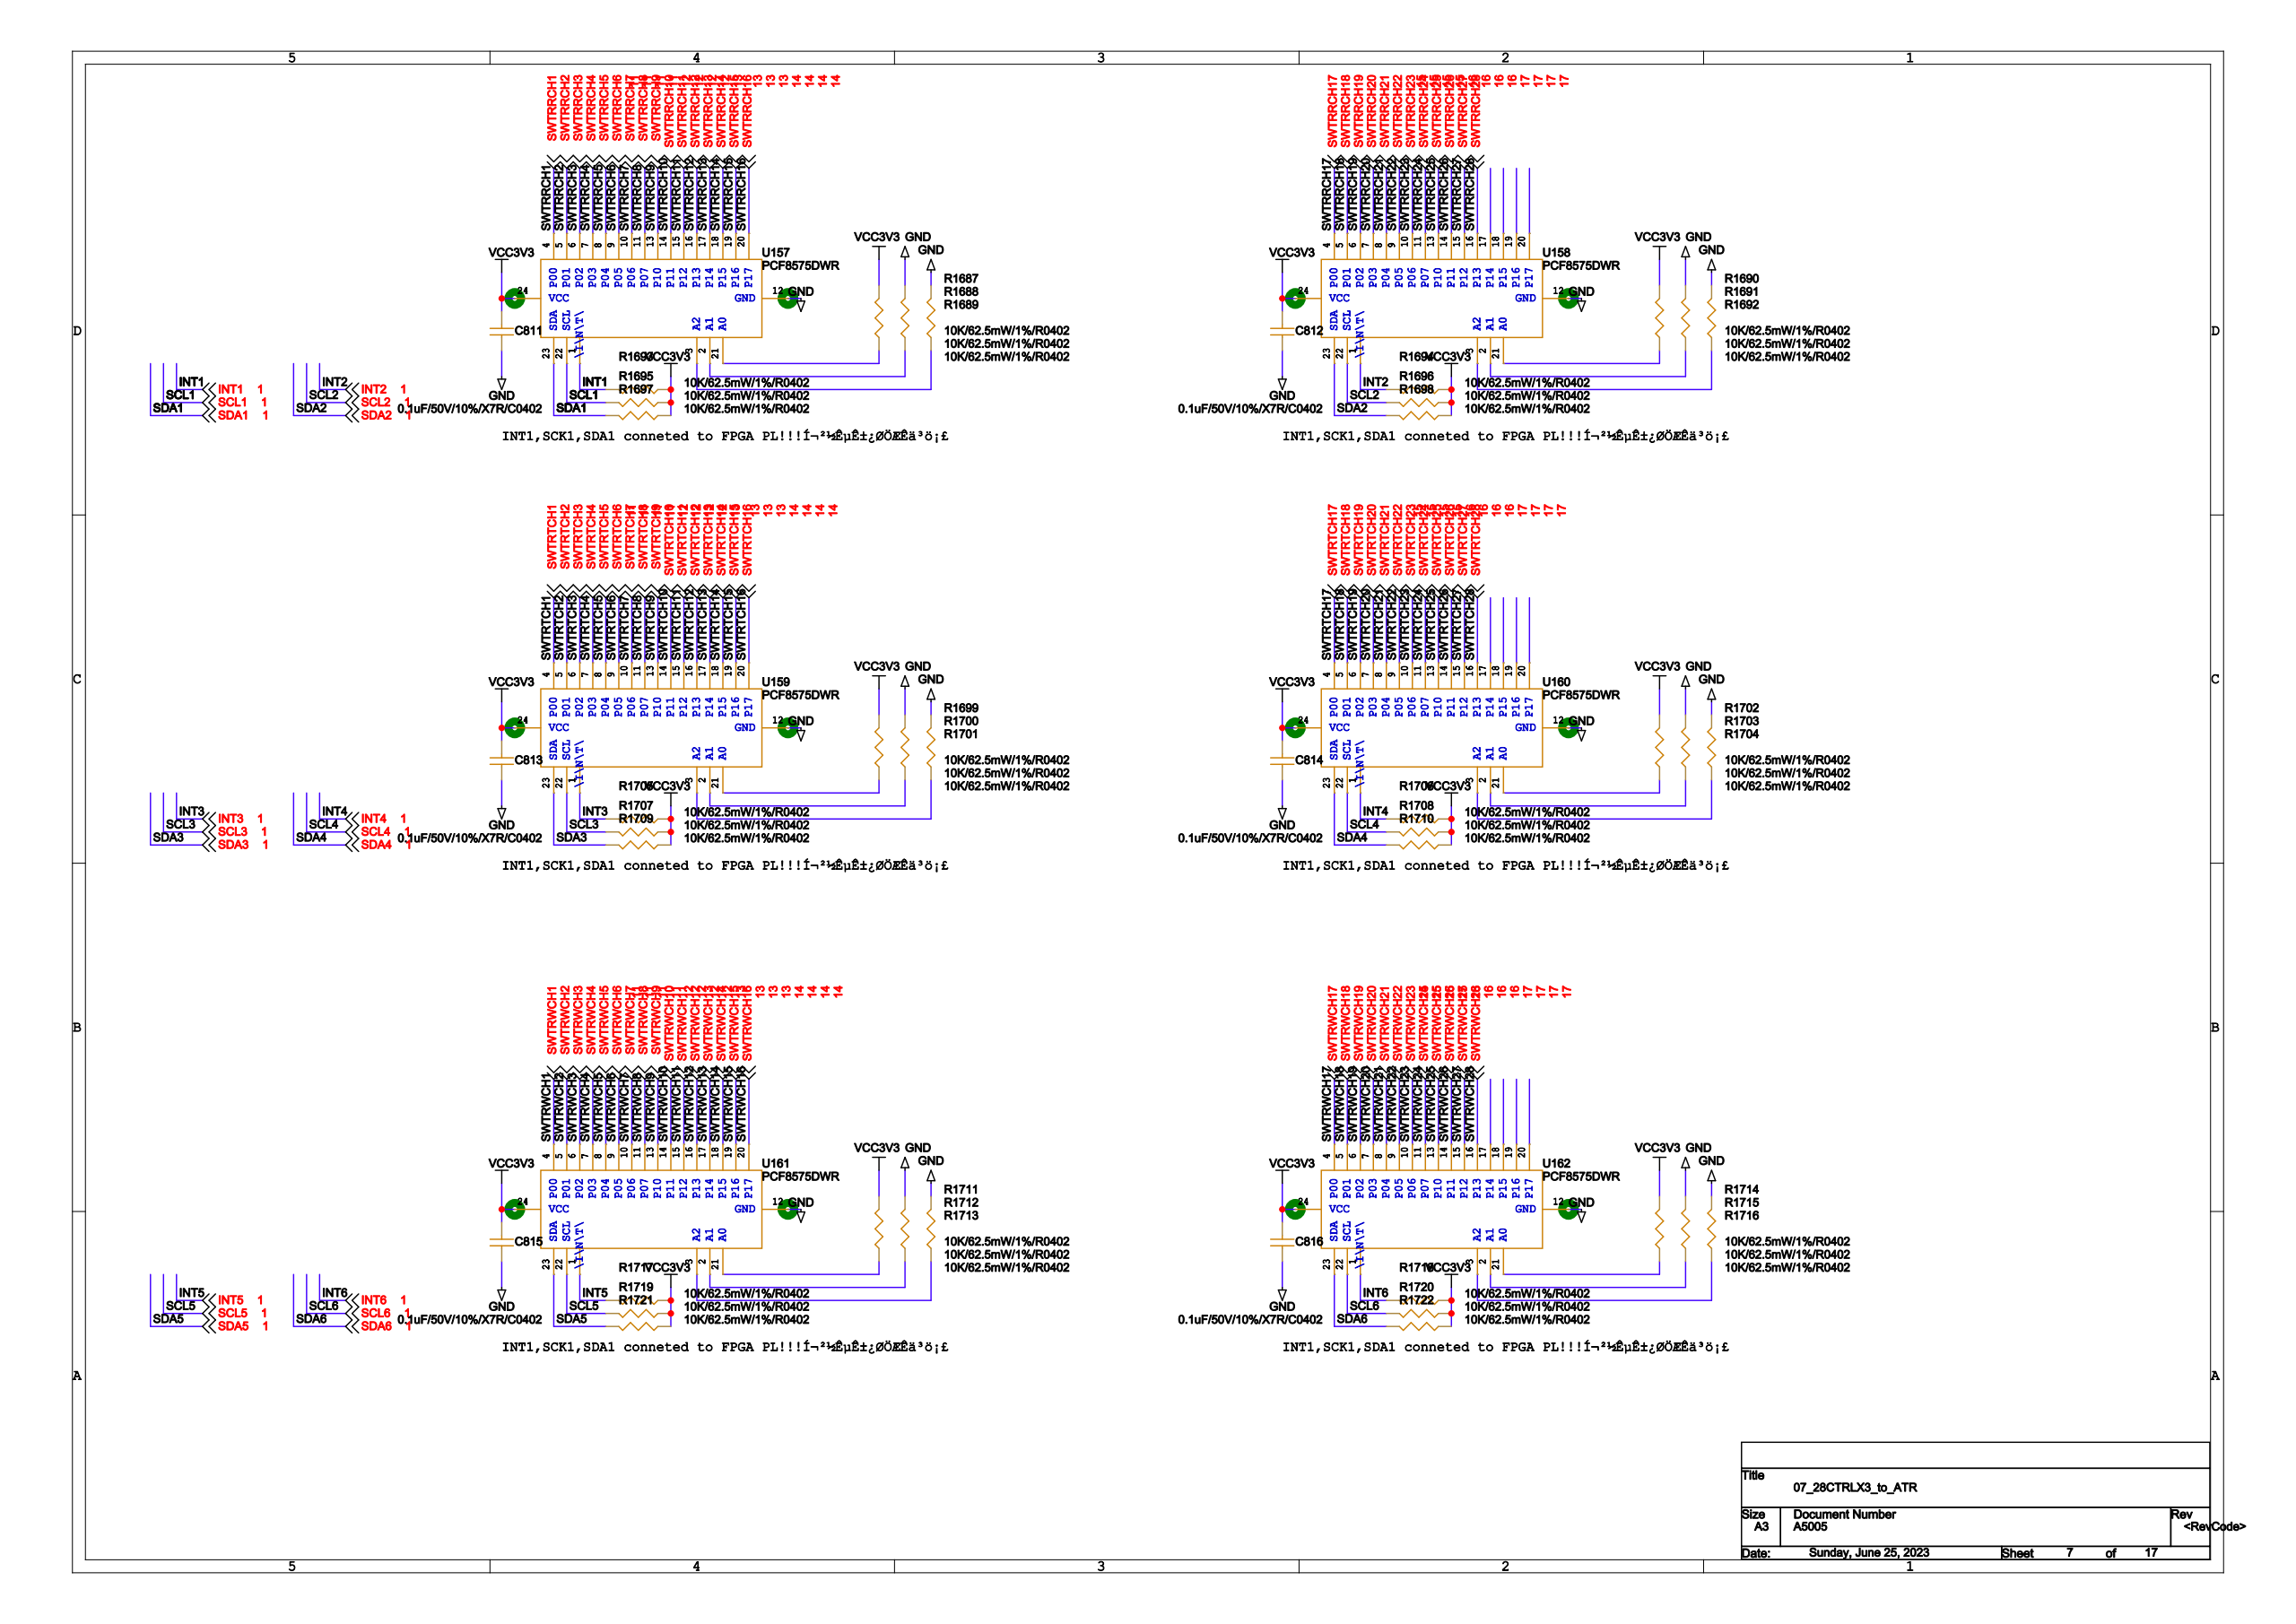Circuit board | Cadence Allegro | 1997 parts | 1536 nets | one sheet of the schematic
Parts on this sheet (reference | value | footprint):
C811 | 0.1uF/50V/10%/X7R/C0402 | 0402
C812 | 0.1uF/50V/10%/X7R/C0402 | 0402
C813 | 0.1uF/50V/10%/X7R/C0402 | 0402
C814 | 0.1uF/50V/10%/X7R/C0402 | 0402
C815 | 0.1uF/50V/10%/X7R/C0402 | 0402
C816 | 0.1uF/50V/10%/X7R/C0402 | 0402
R1687 | 10K/62.5mW/1%/R0402 | 0402
R1688 | 10K/62.5mW/1%/R0402 | 0402
R1689 | 10K/62.5mW/1%/R0402 | 0402
R1690 | 10K/62.5mW/1%/R0402 | 0402
R1691 | 10K/62.5mW/1%/R0402 | 0402
R1692 | 10K/62.5mW/1%/R0402 | 0402
R1693 | 10K/62.5mW/1%/R0402 | 0402
R1694 | 10K/62.5mW/1%/R0402 | 0402
R1695 | 10K/62.5mW/1%/R0402 | 0402
R1696 | 10K/62.5mW/1%/R0402 | 0402
R1697 | 10K/62.5mW/1%/R0402 | 0402
R1698 | 10K/62.5mW/1%/R0402 | 0402
R1699 | 10K/62.5mW/1%/R0402 | 0402
R1700 | 10K/62.5mW/1%/R0402 | 0402
R1701 | 10K/62.5mW/1%/R0402 | 0402
R1702 | 10K/62.5mW/1%/R0402 | 0402
R1703 | 10K/62.5mW/1%/R0402 | 0402
R1704 | 10K/62.5mW/1%/R0402 | 0402
R1705 | 10K/62.5mW/1%/R0402 | 0402
R1706 | 10K/62.5mW/1%/R0402 | 0402
R1707 | 10K/62.5mW/1%/R0402 | 0402
R1708 | 10K/62.5mW/1%/R0402 | 0402
R1709 | 10K/62.5mW/1%/R0402 | 0402
R1710 | 10K/62.5mW/1%/R0402 | 0402
R1711 | 10K/62.5mW/1%/R0402 | 0402
R1712 | 10K/62.5mW/1%/R0402 | 0402
R1713 | 10K/62.5mW/1%/R0402 | 0402
R1714 | 10K/62.5mW/1%/R0402 | 0402
R1715 | 10K/62.5mW/1%/R0402 | 0402
R1716 | 10K/62.5mW/1%/R0402 | 0402
R1717 | 10K/62.5mW/1%/R0402 | 0402
R1718 | 10K/62.5mW/1%/R0402 | 0402
R1719 | 10K/62.5mW/1%/R0402 | 0402
R1720 | 10K/62.5mW/1%/R0402 | 0402
R1721 | 10K/62.5mW/1%/R0402 | 0402
R1722 | 10K/62.5mW/1%/R0402 | 0402
U157 | PCF8575DWR | SOIC_24
U158 | PCF8575DWR | SOIC_24
U159 | PCF8575DWR | SOIC_24
U160 | PCF8575DWR | SOIC_24
U161 | PCF8575DWR | SOIC_24
U162 | PCF8575DWR | SOIC_24
Nets of these parts (net: part-pin ...):
3.3V: C811-2 C812-2 C813-2 C814-2 C815-2 C816-2 R1687-1 R1690-1 R1693-2 R1694-2 R1695-2 R1696-2 R1697-2 R1698-2 R1699-1 R1702-1 R1705-2 R1706-2 R1707-2 R1708-2 R1709-2 R1710-2 R1711-1 R1714-1 R1717-2 R1718-2 R1719-2 R1720-2 R1721-2 R1722-2 U157-24 U158-24 U159-24 U160-24 U161-24 U162-24
AGND: C811-1 C812-1 C813-1 C814-1 C815-1 C816-1 R1688-1 R1689-1 R1691-1 R1692-1 R1700-1 R1701-1 R1703-1 R1704-1 R1712-1 R1713-1 R1715-1 R1716-1 U157-12 U158-12 U159-12 U160-12 U161-12 U162-12
SCL6: R1720-1 U162-22
INT6: R1718-1 U162-1
INT5: R1717-1 U161-1
SDA5: R1721-1 U161-23
SCL5: R1719-1 U161-22
SDA4: R1710-1 U160-23
SCL4: R1708-1 U160-22
INT4: R1706-1 U160-1
SDA3: R1709-1 U159-23
SCL3: R1707-1 U159-22
INT3: R1705-1 U159-1
INT1: R1693-1 U157-1
SDA1: R1697-1 U157-23
SCL1: R1695-1 U157-22
SDA6: R1722-1 U162-23
SDA2: R1698-1 U158-23
SCL2: R1696-1 U158-22
INT2: R1694-1 U158-1
SWTRTCH1: U159-4
SWTRRCH1: U157-4
SWTRWCH1: U161-4
SWTRWCH2: U161-5
SWTRRCH2: U157-5
SWTRTCH2: U159-5
SWTRRCH3: U157-6
SWTRTCH3: U159-6
SWTRWCH3: U161-6
SWTRRCH4: U157-7
SWTRTCH4: U159-7
SWTRWCH4: U161-7
SWTRTCH5: U159-8
SWTRWCH5: U161-8
SWTRRCH5: U157-8
SWTRRCH6: U157-9
SWTRTCH6: U159-9
SWTRWCH6: U161-9
SWTRRCH7: U157-10
SWTRTCH7: U159-10
SWTRWCH7: U161-10
SWTRRCH8: U157-11
SWTRTCH8: U159-11
SWTRWCH8: U161-11
SWTRRCH9: U157-13
SWTRTCH9: U159-13
SWTRWCH9: U161-13
SWTRTCH10: U159-14
SWTRRCH10: U157-14
SWTRWCH10: U161-14
SWTRRCH11: U157-15
SWTRTCH11: U159-15
SWTRWCH11: U161-15
SWTRRCH12: U157-16
SWTRTCH12: U159-16
SWTRWCH12: U161-16
SWTRTCH13: U159-17
SWTRRCH13: U157-17
SWTRWCH13: U161-17
SWTRRCH14: U157-18
SWTRTCH14: U159-18
SWTRWCH14: U161-18
SWTRRCH15: U157-19
SWTRTCH15: U159-19
SWTRWCH15: U161-19
SWTRRCH16: U157-20
SWTRTCH16: U159-20
SWTRWCH16: U161-20
SWTRTCH17: U160-4
SWTRRCH17: U158-4
SWTRWCH17: U162-4
SWTRRCH18: U158-5
SWTRTCH18: U160-5
SWTRWCH18: U162-5
SWTRRCH19: U158-6
SWTRTCH19: U160-6
SWTRWCH19: U162-6
SWTRRCH20: U158-7
SWTRTCH20: U160-7
SWTRWCH20: U162-7
SWTRTCH21: U160-8
SWTRWCH21: U162-8
SWTRRCH21: U158-8
SWTRRCH22: U158-9
SWTRTCH22: U160-9
SWTRWCH22: U162-9
SWTRRCH23: U158-10
SWTRWCH23: U162-10
SWTRTCH23: U160-10
SWTRRCH24: U158-11
SWTRTCH24: U160-11
SWTRWCH24: U162-11
SWTRTCH25: U160-13
SWTRRCH25: U158-13
SWTRWCH25: U162-13
SWTRRCH26: U158-14
SWTRTCH26: U160-14
SWTRWCH26: U162-14
SWTRTCH27: U160-15
SWTRRCH27: U158-15
SWTRWCH27: U162-15
SWTRRCH28: U158-16
SWTRTCH28: U160-16
SWTRWCH28: U162-16
N23855480: R1687-2 U157-21
N23855482: R1688-2 U157-2
N23855484: R1689-2 U157-3
N23856166: R1690-2 U158-21
N23856168: R1691-2 U158-2
N23856170: R1692-2 U158-3
N23988542: R1699-2 U159-21
N23988544: R1700-2 U159-2
N23988546: R1701-2 U159-3
N23988042: R1702-2 U160-21
N23988044: R1703-2 U160-2
N23988046: R1704-2 U160-3
N23990137: R1711-2 U161-21
N23990139: R1712-2 U161-2
N23990141: R1713-2 U161-3
N23989637: R1714-2 U162-21
N23989639: R1715-2 U162-2
N23989641: R1716-2 U162-3